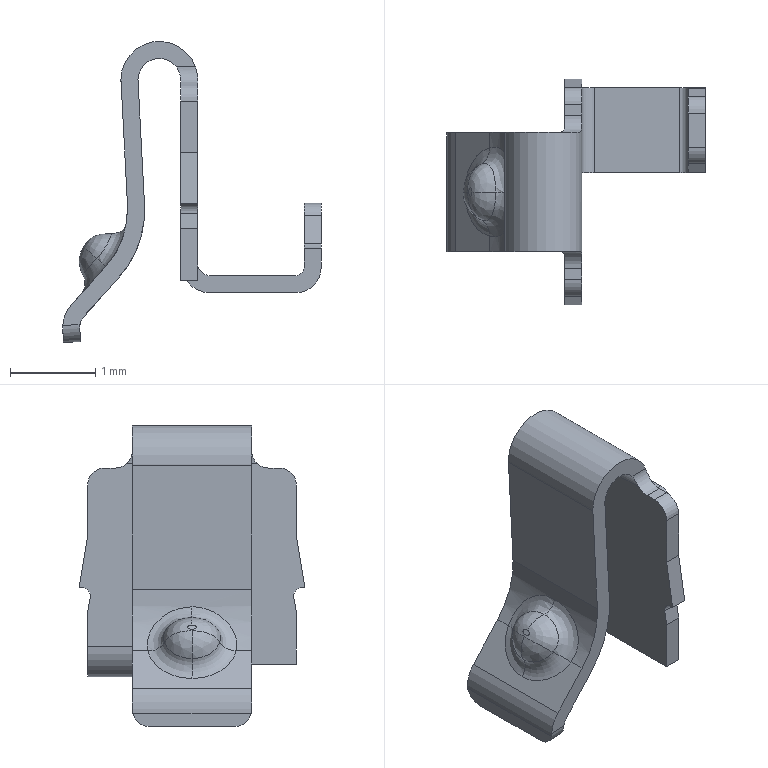Part | Creo | 1 solid | 75 faces | box 3.033 x 2.65 x 3.533 mm | volume 2.841 mm3 | plane 33 | cylinder 26 | spline 12 | torus 4 | commonest cylinder face diameters 0.4 x11 0.2 x3 0.25 x2 0.3 x1 0.5 x1 0.6 x1